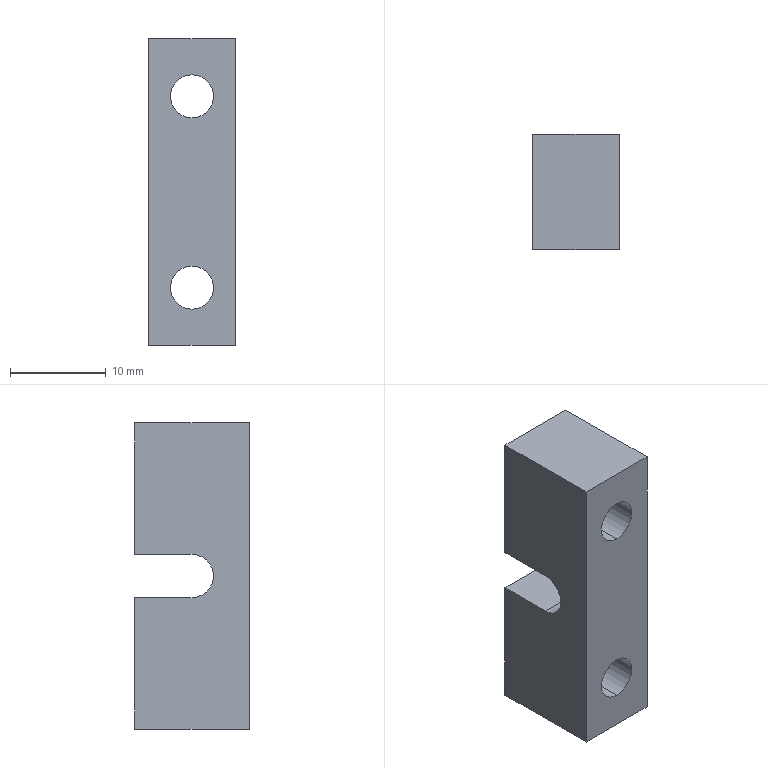Part | STEP file | 001-005-PCB01_5_H6 | 1 solid | 20 faces | box 9 x 12 x 32 mm | volume 2450 mm3 | plane 11 | cylinder 9 | commonest cylinder face diameters 4.5 x5 8 x4
STEP:
#1=CARTESIAN_POINT('',(0.,0.,0.));
#2=DIRECTION('',(0.,0.,1.));
#3=DIRECTION('',(1.,0.,0.));
#4=AXIS2_PLACEMENT_3D('',#1,#2,#3);
#5=CARTESIAN_POINT('',(0.,12.,6.));
#6=VERTEX_POINT('',#5);
#7=CARTESIAN_POINT('',(0.,7.5,6.));
#8=VERTEX_POINT('',#7);
#9=CARTESIAN_POINT('',(0.,12.,6.));
#10=DIRECTION('',(0.,-1.,0.));
#11=VECTOR('',#10,1.);
#12=LINE('',#9,#11);
#13=CARTESIAN_POINT('',(0.,12.,10.));
#14=DIRECTION('',(0.,-1.,0.));
#15=DIRECTION('',(0.,0.,-1.));
#16=AXIS2_PLACEMENT_3D('',#13,#14,#15);
#17=CYLINDRICAL_SURFACE('',#16,4.);
#18=CARTESIAN_POINT('',(6.283,0.));
#19=DIRECTION('',(0.,1.));
#20=VECTOR('',#19,1.);
#21=LINE('',#18,#20);
#22=(GEOMETRIC_REPRESENTATION_CONTEXT(2)PARAMETRIC_REPRESENTATION_CONTEXT()REPRESENTATION_CONTEXT('',''));
#23=DEFINITIONAL_REPRESENTATION('',(#21),#22);
#24=PCURVE('',#17,#23);
#25=CARTESIAN_POINT('',(0.,12.,10.));
#26=DIRECTION('',(0.,-1.,0.));
#27=DIRECTION('',(0.,0.,-1.));
#28=AXIS2_PLACEMENT_3D('',#25,#26,#27);
#29=CYLINDRICAL_SURFACE('',#28,4.);
#30=CARTESIAN_POINT('',(0.,0.));
#31=DIRECTION('',(0.,1.));
#32=VECTOR('',#31,1.);
#33=LINE('',#30,#32);
#34=(GEOMETRIC_REPRESENTATION_CONTEXT(2)PARAMETRIC_REPRESENTATION_CONTEXT()REPRESENTATION_CONTEXT('',''));
#35=DEFINITIONAL_REPRESENTATION('',(#33),#34);
#36=PCURVE('',#29,#35);
#37=SURFACE_CURVE('',#12,(#24,#36),.PCURVE_S1.);
#38=EDGE_CURVE('',#6,#8,#37,.T.);
#39=ORIENTED_EDGE('',*,*,#38,.T.);
#40=CARTESIAN_POINT('',(0.,7.5,14.));
#41=VERTEX_POINT('',#40);
#42=CARTESIAN_POINT('',(0.,7.5,10.));
#43=DIRECTION('',(0.,-1.,0.));
#44=DIRECTION('',(0.,0.,-1.));
#45=AXIS2_PLACEMENT_3D('',#42,#43,#44);
#46=CIRCLE('',#45,4.);
#47=CARTESIAN_POINT('',(0.,4.5));
#48=DIRECTION('',(1.,0.));
#49=VECTOR('',#48,1.);
#50=LINE('',#47,#49);
#51=(GEOMETRIC_REPRESENTATION_CONTEXT(2)PARAMETRIC_REPRESENTATION_CONTEXT()REPRESENTATION_CONTEXT('',''));
#52=DEFINITIONAL_REPRESENTATION('',(#50),#51);
#53=PCURVE('',#17,#52);
#54=CARTESIAN_POINT('',(0.,7.5,12.25));
#55=DIRECTION('',(0.,1.,0.));
#56=DIRECTION('',(0.,0.,1.));
#57=AXIS2_PLACEMENT_3D('',#54,#55,#56);
#58=PLANE('',#57);
#59=CARTESIAN_POINT('',(-6.25,0.));
#60=CARTESIAN_POINT('',(-6.25,6.928));
#61=CARTESIAN_POINT('',(-0.25,3.464));
#62=CARTESIAN_POINT('',(5.75,0.));
#63=CARTESIAN_POINT('',(-0.25,-3.464));
#64=CARTESIAN_POINT('',(-6.25,-6.928));
#65=CARTESIAN_POINT('',(-6.25,0.));
#66=(BOUNDED_CURVE()B_SPLINE_CURVE(2,(#59,#60,#61,#62,#63,#64,#65),.UNSPECIFIED.,.T.,.F.)B_SPLINE_CURVE_WITH_KNOTS((1,2,2,2,2,1),(-2.094,0.,2.094,4.189,6.283,8.378),.UNSPECIFIED.)CURVE()GEOMETRIC_REPRESENTATION_ITEM()RATIONAL_B_SPLINE_CURVE((1.,0.5,1.,0.5,1.,0.5,1.))REPRESENTATION_ITEM(''));
#67=(GEOMETRIC_REPRESENTATION_CONTEXT(2)PARAMETRIC_REPRESENTATION_CONTEXT()REPRESENTATION_CONTEXT('',''));
#68=DEFINITIONAL_REPRESENTATION('',(#66),#67);
#69=PCURVE('',#58,#68);
#70=SURFACE_CURVE('',#46,(#53,#69),.PCURVE_S1.);
#71=EDGE_CURVE('',#41,#8,#70,.T.);
#72=ORIENTED_EDGE('',*,*,#71,.F.);
#73=CARTESIAN_POINT('',(0.,12.,14.));
#74=VERTEX_POINT('',#73);
#75=CARTESIAN_POINT('',(0.,12.,14.));
#76=DIRECTION('',(0.,-1.,0.));
#77=VECTOR('',#76,1.);
#78=LINE('',#75,#77);
#79=CARTESIAN_POINT('',(3.142,0.));
#80=DIRECTION('',(0.,1.));
#81=VECTOR('',#80,1.);
#82=LINE('',#79,#81);
#83=(GEOMETRIC_REPRESENTATION_CONTEXT(2)PARAMETRIC_REPRESENTATION_CONTEXT()REPRESENTATION_CONTEXT('',''));
#84=DEFINITIONAL_REPRESENTATION('',(#82),#83);
#85=PCURVE('',#17,#84);
#86=CARTESIAN_POINT('',(3.142,0.));
#87=DIRECTION('',(0.,1.));
#88=VECTOR('',#87,1.);
#89=LINE('',#86,#88);
#90=(GEOMETRIC_REPRESENTATION_CONTEXT(2)PARAMETRIC_REPRESENTATION_CONTEXT()REPRESENTATION_CONTEXT('',''));
#91=DEFINITIONAL_REPRESENTATION('',(#89),#90);
#92=PCURVE('',#29,#91);
#93=SURFACE_CURVE('',#78,(#85,#92),.PCURVE_S1.);
#94=EDGE_CURVE('',#74,#41,#93,.T.);
#95=ORIENTED_EDGE('',*,*,#94,.F.);
#96=CARTESIAN_POINT('',(0.,12.,10.));
#97=DIRECTION('',(0.,-1.,0.));
#98=DIRECTION('',(0.,0.,-1.));
#99=AXIS2_PLACEMENT_3D('',#96,#97,#98);
#100=CIRCLE('',#99,4.);
#101=CARTESIAN_POINT('',(0.,0.));
#102=DIRECTION('',(1.,0.));
#103=VECTOR('',#102,1.);
#104=LINE('',#101,#103);
#105=(GEOMETRIC_REPRESENTATION_CONTEXT(2)PARAMETRIC_REPRESENTATION_CONTEXT()REPRESENTATION_CONTEXT('',''));
#106=DEFINITIONAL_REPRESENTATION('',(#104),#105);
#107=PCURVE('',#17,#106);
#108=CARTESIAN_POINT('',(4.5,12.,2.25));
#109=DIRECTION('',(0.,-1.,0.));
#110=DIRECTION('',(0.,0.,-1.));
#111=AXIS2_PLACEMENT_3D('',#108,#109,#110);
#112=PLANE('',#111);
#113=CARTESIAN_POINT('',(-7.75,-4.5));
#114=DIRECTION('',(1.,0.));
#115=AXIS2_PLACEMENT_2D('',#113,#114);
#116=CIRCLE('',#115,4.);
#117=(GEOMETRIC_REPRESENTATION_CONTEXT(2)PARAMETRIC_REPRESENTATION_CONTEXT()REPRESENTATION_CONTEXT('',''));
#118=DEFINITIONAL_REPRESENTATION('',(#116),#117);
#119=PCURVE('',#112,#118);
#120=SURFACE_CURVE('',#100,(#107,#119),.PCURVE_S1.);
#121=EDGE_CURVE('',#74,#6,#120,.T.);
#122=ORIENTED_EDGE('',*,*,#121,.T.);
#123=EDGE_LOOP('',(#39,#72,#95,#122));
#124=FACE_BOUND('',#123,.F.);
#125=ADVANCED_FACE('',(#124),#17,.F.);
#126=CARTESIAN_POINT('',(0.,7.5,7.75));
#127=VERTEX_POINT('',#126);
#128=CARTESIAN_POINT('',(0.,0.,7.75));
#129=VERTEX_POINT('',#128);
#130=CARTESIAN_POINT('',(0.,12.,7.75));
#131=DIRECTION('',(0.,-1.,0.));
#132=VECTOR('',#131,1.);
#133=LINE('',#130,#132);
#134=CARTESIAN_POINT('',(0.,12.,10.));
#135=DIRECTION('',(0.,-1.,0.));
#136=DIRECTION('',(0.,0.,-1.));
#137=AXIS2_PLACEMENT_3D('',#134,#135,#136);
#138=CYLINDRICAL_SURFACE('',#137,2.25);
#139=CARTESIAN_POINT('',(6.283,0.));
#140=DIRECTION('',(0.,1.));
#141=VECTOR('',#140,1.);
#142=LINE('',#139,#141);
#143=(GEOMETRIC_REPRESENTATION_CONTEXT(2)PARAMETRIC_REPRESENTATION_CONTEXT()REPRESENTATION_CONTEXT('',''));
#144=DEFINITIONAL_REPRESENTATION('',(#142),#143);
#145=PCURVE('',#138,#144);
#146=CARTESIAN_POINT('',(0.,12.,10.));
#147=DIRECTION('',(0.,-1.,0.));
#148=DIRECTION('',(0.,0.,-1.));
#149=AXIS2_PLACEMENT_3D('',#146,#147,#148);
#150=CYLINDRICAL_SURFACE('',#149,2.25);
#151=CARTESIAN_POINT('',(0.,0.));
#152=DIRECTION('',(0.,1.));
#153=VECTOR('',#152,1.);
#154=LINE('',#151,#153);
#155=(GEOMETRIC_REPRESENTATION_CONTEXT(2)PARAMETRIC_REPRESENTATION_CONTEXT()REPRESENTATION_CONTEXT('',''));
#156=DEFINITIONAL_REPRESENTATION('',(#154),#155);
#157=PCURVE('',#150,#156);
#158=SURFACE_CURVE('',#133,(#145,#157),.PCURVE_S1.);
#159=EDGE_CURVE('',#127,#129,#158,.T.);
#160=ORIENTED_EDGE('',*,*,#159,.T.);
#161=CARTESIAN_POINT('',(0.,0.,12.25));
#162=VERTEX_POINT('',#161);
#163=CARTESIAN_POINT('',(0.,0.,10.));
#164=DIRECTION('',(0.,-1.,0.));
#165=DIRECTION('',(0.,0.,-1.));
#166=AXIS2_PLACEMENT_3D('',#163,#164,#165);
#167=CIRCLE('',#166,2.25);
#168=CARTESIAN_POINT('',(0.,12.));
#169=DIRECTION('',(1.,0.));
#170=VECTOR('',#169,1.);
#171=LINE('',#168,#170);
#172=(GEOMETRIC_REPRESENTATION_CONTEXT(2)PARAMETRIC_REPRESENTATION_CONTEXT()REPRESENTATION_CONTEXT('',''));
#173=DEFINITIONAL_REPRESENTATION('',(#171),#172);
#174=PCURVE('',#138,#173);
#175=CARTESIAN_POINT('',(4.5,0.,16.));
#176=DIRECTION('',(0.,1.,0.));
#177=DIRECTION('',(0.,0.,1.));
#178=AXIS2_PLACEMENT_3D('',#175,#176,#177);
#179=PLANE('',#178);
#180=CARTESIAN_POINT('',(-8.25,-4.5));
#181=CARTESIAN_POINT('',(-8.25,-0.6029));
#182=CARTESIAN_POINT('',(-4.875,-2.551));
#183=CARTESIAN_POINT('',(-1.5,-4.5));
#184=CARTESIAN_POINT('',(-4.875,-6.449));
#185=CARTESIAN_POINT('',(-8.25,-8.397));
#186=CARTESIAN_POINT('',(-8.25,-4.5));
#187=(BOUNDED_CURVE()B_SPLINE_CURVE(2,(#180,#181,#182,#183,#184,#185,#186),.UNSPECIFIED.,.T.,.F.)B_SPLINE_CURVE_WITH_KNOTS((1,2,2,2,2,1),(-2.094,0.,2.094,4.189,6.283,8.378),.UNSPECIFIED.)CURVE()GEOMETRIC_REPRESENTATION_ITEM()RATIONAL_B_SPLINE_CURVE((1.,0.5,1.,0.5,1.,0.5,1.))REPRESENTATION_ITEM(''));
#188=(GEOMETRIC_REPRESENTATION_CONTEXT(2)PARAMETRIC_REPRESENTATION_CONTEXT()REPRESENTATION_CONTEXT('',''));
#189=DEFINITIONAL_REPRESENTATION('',(#187),#188);
#190=PCURVE('',#179,#189);
#191=SURFACE_CURVE('',#167,(#174,#190),.PCURVE_S1.);
#192=EDGE_CURVE('',#162,#129,#191,.T.);
#193=ORIENTED_EDGE('',*,*,#192,.F.);
#194=CARTESIAN_POINT('',(0.,7.5,12.25));
#195=VERTEX_POINT('',#194);
#196=CARTESIAN_POINT('',(0.,12.,12.25));
#197=DIRECTION('',(0.,-1.,0.));
#198=VECTOR('',#197,1.);
#199=LINE('',#196,#198);
#200=CARTESIAN_POINT('',(3.142,0.));
#201=DIRECTION('',(0.,1.));
#202=VECTOR('',#201,1.);
#203=LINE('',#200,#202);
#204=(GEOMETRIC_REPRESENTATION_CONTEXT(2)PARAMETRIC_REPRESENTATION_CONTEXT()REPRESENTATION_CONTEXT('',''));
#205=DEFINITIONAL_REPRESENTATION('',(#203),#204);
#206=PCURVE('',#138,#205);
#207=CARTESIAN_POINT('',(3.142,0.));
#208=DIRECTION('',(0.,1.));
#209=VECTOR('',#208,1.);
#210=LINE('',#207,#209);
#211=(GEOMETRIC_REPRESENTATION_CONTEXT(2)PARAMETRIC_REPRESENTATION_CONTEXT()REPRESENTATION_CONTEXT('',''));
#212=DEFINITIONAL_REPRESENTATION('',(#210),#211);
#213=PCURVE('',#150,#212);
#214=SURFACE_CURVE('',#199,(#206,#213),.PCURVE_S1.);
#215=EDGE_CURVE('',#195,#162,#214,.T.);
#216=ORIENTED_EDGE('',*,*,#215,.F.);
#217=CARTESIAN_POINT('',(0.,7.5,10.));
#218=DIRECTION('',(0.,-1.,0.));
#219=DIRECTION('',(0.,0.,-1.));
#220=AXIS2_PLACEMENT_3D('',#217,#218,#219);
#221=CIRCLE('',#220,2.25);
#222=CARTESIAN_POINT('',(0.,4.5));
#223=DIRECTION('',(1.,0.));
#224=VECTOR('',#223,1.);
#225=LINE('',#222,#224);
#226=(GEOMETRIC_REPRESENTATION_CONTEXT(2)PARAMETRIC_REPRESENTATION_CONTEXT()REPRESENTATION_CONTEXT('',''));
#227=DEFINITIONAL_REPRESENTATION('',(#225),#226);
#228=PCURVE('',#138,#227);
#229=CARTESIAN_POINT('',(-4.5,0.));
#230=CARTESIAN_POINT('',(-4.5,3.897));
#231=CARTESIAN_POINT('',(-1.125,1.949));
#232=CARTESIAN_POINT('',(2.25,0.));
#233=CARTESIAN_POINT('',(-1.125,-1.949));
#234=CARTESIAN_POINT('',(-4.5,-3.897));
#235=CARTESIAN_POINT('',(-4.5,0.));
#236=(BOUNDED_CURVE()B_SPLINE_CURVE(2,(#229,#230,#231,#232,#233,#234,#235),.UNSPECIFIED.,.T.,.F.)B_SPLINE_CURVE_WITH_KNOTS((1,2,2,2,2,1),(-2.094,0.,2.094,4.189,6.283,8.378),.UNSPECIFIED.)CURVE()GEOMETRIC_REPRESENTATION_ITEM()RATIONAL_B_SPLINE_CURVE((1.,0.5,1.,0.5,1.,0.5,1.))REPRESENTATION_ITEM(''));
#237=(GEOMETRIC_REPRESENTATION_CONTEXT(2)PARAMETRIC_REPRESENTATION_CONTEXT()REPRESENTATION_CONTEXT('',''));
#238=DEFINITIONAL_REPRESENTATION('',(#236),#237);
#239=PCURVE('',#58,#238);
#240=SURFACE_CURVE('',#221,(#228,#239),.PCURVE_S1.);
#241=EDGE_CURVE('',#195,#127,#240,.T.);
#242=ORIENTED_EDGE('',*,*,#241,.T.);
#243=EDGE_LOOP('',(#160,#193,#216,#242));
#244=FACE_BOUND('',#243,.F.);
#245=ADVANCED_FACE('',(#244),#138,.F.);
#246=CARTESIAN_POINT('',(0.,12.,-14.));
#247=VERTEX_POINT('',#246);
#248=CARTESIAN_POINT('',(0.,7.5,-14.));
#249=VERTEX_POINT('',#248);
#250=CARTESIAN_POINT('',(0.,12.,-14.));
#251=DIRECTION('',(0.,-1.,0.));
#252=VECTOR('',#251,1.);
#253=LINE('',#250,#252);
#254=CARTESIAN_POINT('',(0.,12.,-10.));
#255=DIRECTION('',(0.,-1.,0.));
#256=DIRECTION('',(0.,0.,-1.));
#257=AXIS2_PLACEMENT_3D('',#254,#255,#256);
#258=CYLINDRICAL_SURFACE('',#257,4.);
#259=CARTESIAN_POINT('',(6.283,0.));
#260=DIRECTION('',(0.,1.));
#261=VECTOR('',#260,1.);
#262=LINE('',#259,#261);
#263=(GEOMETRIC_REPRESENTATION_CONTEXT(2)PARAMETRIC_REPRESENTATION_CONTEXT()REPRESENTATION_CONTEXT('',''));
#264=DEFINITIONAL_REPRESENTATION('',(#262),#263);
#265=PCURVE('',#258,#264);
#266=CARTESIAN_POINT('',(0.,12.,-10.));
#267=DIRECTION('',(0.,-1.,0.));
#268=DIRECTION('',(0.,0.,-1.));
#269=AXIS2_PLACEMENT_3D('',#266,#267,#268);
#270=CYLINDRICAL_SURFACE('',#269,4.);
#271=CARTESIAN_POINT('',(0.,0.));
#272=DIRECTION('',(0.,1.));
#273=VECTOR('',#272,1.);
#274=LINE('',#271,#273);
#275=(GEOMETRIC_REPRESENTATION_CONTEXT(2)PARAMETRIC_REPRESENTATION_CONTEXT()REPRESENTATION_CONTEXT('',''));
#276=DEFINITIONAL_REPRESENTATION('',(#274),#275);
#277=PCURVE('',#270,#276);
#278=SURFACE_CURVE('',#253,(#265,#277),.PCURVE_S1.);
#279=EDGE_CURVE('',#247,#249,#278,.T.);
#280=ORIENTED_EDGE('',*,*,#279,.T.);
#281=CARTESIAN_POINT('',(0.,7.5,-6.));
#282=VERTEX_POINT('',#281);
#283=CARTESIAN_POINT('',(0.,7.5,-10.));
#284=DIRECTION('',(0.,-1.,0.));
#285=DIRECTION('',(0.,0.,-1.));
#286=AXIS2_PLACEMENT_3D('',#283,#284,#285);
#287=CIRCLE('',#286,4.);
#288=CARTESIAN_POINT('',(0.,4.5));
#289=DIRECTION('',(1.,0.));
#290=VECTOR('',#289,1.);
#291=LINE('',#288,#290);
#292=(GEOMETRIC_REPRESENTATION_CONTEXT(2)PARAMETRIC_REPRESENTATION_CONTEXT()REPRESENTATION_CONTEXT('',''));
#293=DEFINITIONAL_REPRESENTATION('',(#291),#292);
#294=PCURVE('',#258,#293);
#295=CARTESIAN_POINT('',(0.,7.5,-7.75));
#296=DIRECTION('',(0.,1.,0.));
#297=DIRECTION('',(0.,0.,1.));
#298=AXIS2_PLACEMENT_3D('',#295,#296,#297);
#299=PLANE('',#298);
#300=CARTESIAN_POINT('',(-6.25,0.));
#301=CARTESIAN_POINT('',(-6.25,6.928));
#302=CARTESIAN_POINT('',(-0.25,3.464));
#303=CARTESIAN_POINT('',(5.75,0.));
#304=CARTESIAN_POINT('',(-0.25,-3.464));
#305=CARTESIAN_POINT('',(-6.25,-6.928));
#306=CARTESIAN_POINT('',(-6.25,0.));
#307=(BOUNDED_CURVE()B_SPLINE_CURVE(2,(#300,#301,#302,#303,#304,#305,#306),.UNSPECIFIED.,.T.,.F.)B_SPLINE_CURVE_WITH_KNOTS((1,2,2,2,2,1),(-2.094,0.,2.094,4.189,6.283,8.378),.UNSPECIFIED.)CURVE()GEOMETRIC_REPRESENTATION_ITEM()RATIONAL_B_SPLINE_CURVE((1.,0.5,1.,0.5,1.,0.5,1.))REPRESENTATION_ITEM(''));
#308=(GEOMETRIC_REPRESENTATION_CONTEXT(2)PARAMETRIC_REPRESENTATION_CONTEXT()REPRESENTATION_CONTEXT('',''));
#309=DEFINITIONAL_REPRESENTATION('',(#307),#308);
#310=PCURVE('',#299,#309);
#311=SURFACE_CURVE('',#287,(#294,#310),.PCURVE_S1.);
#312=EDGE_CURVE('',#282,#249,#311,.T.);
#313=ORIENTED_EDGE('',*,*,#312,.F.);
#314=CARTESIAN_POINT('',(0.,12.,-6.));
#315=VERTEX_POINT('',#314);
#316=CARTESIAN_POINT('',(0.,12.,-6.));
#317=DIRECTION('',(0.,-1.,0.));
#318=VECTOR('',#317,1.);
#319=LINE('',#316,#318);
#320=CARTESIAN_POINT('',(3.142,0.));
#321=DIRECTION('',(0.,1.));
#322=VECTOR('',#321,1.);
#323=LINE('',#320,#322);
#324=(GEOMETRIC_REPRESENTATION_CONTEXT(2)PARAMETRIC_REPRESENTATION_CONTEXT()REPRESENTATION_CONTEXT('',''));
#325=DEFINITIONAL_REPRESENTATION('',(#323),#324);
#326=PCURVE('',#258,#325);
#327=CARTESIAN_POINT('',(3.142,0.));
#328=DIRECTION('',(0.,1.));
#329=VECTOR('',#328,1.);
#330=LINE('',#327,#329);
#331=(GEOMETRIC_REPRESENTATION_CONTEXT(2)PARAMETRIC_REPRESENTATION_CONTEXT()REPRESENTATION_CONTEXT('',''));
#332=DEFINITIONAL_REPRESENTATION('',(#330),#331);
#333=PCURVE('',#270,#332);
#334=SURFACE_CURVE('',#319,(#326,#333),.PCURVE_S1.);
#335=EDGE_CURVE('',#315,#282,#334,.T.);
#336=ORIENTED_EDGE('',*,*,#335,.F.);
#337=CARTESIAN_POINT('',(0.,12.,-10.));
#338=DIRECTION('',(0.,-1.,0.));
#339=DIRECTION('',(0.,0.,-1.));
#340=AXIS2_PLACEMENT_3D('',#337,#338,#339);
#341=CIRCLE('',#340,4.);
#342=CARTESIAN_POINT('',(0.,0.));
#343=DIRECTION('',(1.,0.));
#344=VECTOR('',#343,1.);
#345=LINE('',#342,#344);
#346=(GEOMETRIC_REPRESENTATION_CONTEXT(2)PARAMETRIC_REPRESENTATION_CONTEXT()REPRESENTATION_CONTEXT('',''));
#347=DEFINITIONAL_REPRESENTATION('',(#345),#346);
#348=PCURVE('',#258,#347);
#349=CARTESIAN_POINT('',(4.5,12.,-16.));
#350=DIRECTION('',(0.,-1.,0.));
#351=DIRECTION('',(0.,0.,-1.));
#352=AXIS2_PLACEMENT_3D('',#349,#350,#351);
#353=PLANE('',#352);
#354=CARTESIAN_POINT('',(-6.,-4.5));
#355=DIRECTION('',(1.,0.));
#356=AXIS2_PLACEMENT_2D('',#354,#355);
#357=CIRCLE('',#356,4.);
#358=(GEOMETRIC_REPRESENTATION_CONTEXT(2)PARAMETRIC_REPRESENTATION_CONTEXT()REPRESENTATION_CONTEXT('',''));
#359=DEFINITIONAL_REPRESENTATION('',(#357),#358);
#360=PCURVE('',#353,#359);
#361=SURFACE_CURVE('',#341,(#348,#360),.PCURVE_S1.);
#362=EDGE_CURVE('',#315,#247,#361,.T.);
#363=ORIENTED_EDGE('',*,*,#362,.T.);
#364=EDGE_LOOP('',(#280,#313,#336,#363));
#365=FACE_BOUND('',#364,.F.);
#366=ADVANCED_FACE('',(#365),#258,.F.);
#367=CARTESIAN_POINT('',(0.,7.5,-12.25));
#368=VERTEX_POINT('',#367);
#369=CARTESIAN_POINT('',(0.,0.,-12.25));
#370=VERTEX_POINT('',#369);
#371=CARTESIAN_POINT('',(0.,12.,-12.25));
#372=DIRECTION('',(0.,-1.,0.));
#373=VECTOR('',#372,1.);
#374=LINE('',#371,#373);
#375=CARTESIAN_POINT('',(0.,12.,-10.));
#376=DIRECTION('',(0.,-1.,0.));
#377=DIRECTION('',(0.,0.,-1.));
#378=AXIS2_PLACEMENT_3D('',#375,#376,#377);
#379=CYLINDRICAL_SURFACE('',#378,2.25);
#380=CARTESIAN_POINT('',(6.283,0.));
#381=DIRECTION('',(0.,1.));
#382=VECTOR('',#381,1.);
#383=LINE('',#380,#382);
#384=(GEOMETRIC_REPRESENTATION_CONTEXT(2)PARAMETRIC_REPRESENTATION_CONTEXT()REPRESENTATION_CONTEXT('',''));
#385=DEFINITIONAL_REPRESENTATION('',(#383),#384);
#386=PCURVE('',#379,#385);
#387=CARTESIAN_POINT('',(0.,12.,-10.));
#388=DIRECTION('',(0.,-1.,0.));
#389=DIRECTION('',(0.,0.,-1.));
#390=AXIS2_PLACEMENT_3D('',#387,#388,#389);
#391=CYLINDRICAL_SURFACE('',#390,2.25);
#392=CARTESIAN_POINT('',(0.,0.));
#393=DIRECTION('',(0.,1.));
#394=VECTOR('',#393,1.);
#395=LINE('',#392,#394);
#396=(GEOMETRIC_REPRESENTATION_CONTEXT(2)PARAMETRIC_REPRESENTATION_CONTEXT()REPRESENTATION_CONTEXT('',''));
#397=DEFINITIONAL_REPRESENTATION('',(#395),#396);
#398=PCURVE('',#391,#397);
#399=SURFACE_CURVE('',#374,(#386,#398),.PCURVE_S1.);
#400=EDGE_CURVE('',#368,#370,#399,.T.);
#401=ORIENTED_EDGE('',*,*,#400,.T.);
#402=CARTESIAN_POINT('',(0.,0.,-7.75));
#403=VERTEX_POINT('',#402);
#404=CARTESIAN_POINT('',(0.,0.,-10.));
#405=DIRECTION('',(0.,-1.,0.));
#406=DIRECTION('',(0.,0.,-1.));
#407=AXIS2_PLACEMENT_3D('',#404,#405,#406);
#408=CIRCLE('',#407,2.25);
#409=CARTESIAN_POINT('',(0.,12.));
#410=DIRECTION('',(1.,0.));
#411=VECTOR('',#410,1.);
#412=LINE('',#409,#411);
#413=(GEOMETRIC_REPRESENTATION_CONTEXT(2)PARAMETRIC_REPRESENTATION_CONTEXT()REPRESENTATION_CONTEXT('',''));
#414=DEFINITIONAL_REPRESENTATION('',(#412),#413);
#415=PCURVE('',#379,#414);
#416=CARTESIAN_POINT('',(-28.25,-4.5));
#417=CARTESIAN_POINT('',(-28.25,-0.6029));
#418=CARTESIAN_POINT('',(-24.875,-2.551));
#419=CARTESIAN_POINT('',(-21.5,-4.5));
#420=CARTESIAN_POINT('',(-24.875,-6.449));
#421=CARTESIAN_POINT('',(-28.25,-8.397));
#422=CARTESIAN_POINT('',(-28.25,-4.5));
#423=(BOUNDED_CURVE()B_SPLINE_CURVE(2,(#416,#417,#418,#419,#420,#421,#422),.UNSPECIFIED.,.T.,.F.)B_SPLINE_CURVE_WITH_KNOTS((1,2,2,2,2,1),(-2.094,0.,2.094,4.189,6.283,8.378),.UNSPECIFIED.)CURVE()GEOMETRIC_REPRESENTATION_ITEM()RATIONAL_B_SPLINE_CURVE((1.,0.5,1.,0.5,1.,0.5,1.))REPRESENTATION_ITEM(''));
#424=(GEOMETRIC_REPRESENTATION_CONTEXT(2)PARAMETRIC_REPRESENTATION_CONTEXT()REPRESENTATION_CONTEXT('',''));
#425=DEFINITIONAL_REPRESENTATION('',(#423),#424);
#426=PCURVE('',#179,#425);
#427=SURFACE_CURVE('',#408,(#415,#426),.PCURVE_S1.);
#428=EDGE_CURVE('',#403,#370,#427,.T.);
#429=ORIENTED_EDGE('',*,*,#428,.F.);
#430=CARTESIAN_POINT('',(0.,7.5,-7.75));
#431=VERTEX_POINT('',#430);
#432=CARTESIAN_POINT('',(0.,12.,-7.75));
#433=DIRECTION('',(0.,-1.,0.));
#434=VECTOR('',#433,1.);
#435=LINE('',#432,#434);
#436=CARTESIAN_POINT('',(3.142,0.));
#437=DIRECTION('',(0.,1.));
#438=VECTOR('',#437,1.);
#439=LINE('',#436,#438);
#440=(GEOMETRIC_REPRESENTATION_CONTEXT(2)PARAMETRIC_REPRESENTATION_CONTEXT()REPRESENTATION_CONTEXT('',''));
#441=DEFINITIONAL_REPRESENTATION('',(#439),#440);
#442=PCURVE('',#379,#441);
#443=CARTESIAN_POINT('',(3.142,0.));
#444=DIRECTION('',(0.,1.));
#445=VECTOR('',#444,1.);
#446=LINE('',#443,#445);
#447=(GEOMETRIC_REPRESENTATION_CONTEXT(2)PARAMETRIC_REPRESENTATION_CONTEXT()REPRESENTATION_CONTEXT('',''));
#448=DEFINITIONAL_REPRESENTATION('',(#446),#447);
#449=PCURVE('',#391,#448);
#450=SURFACE_CURVE('',#435,(#442,#449),.PCURVE_S1.);
#451=EDGE_CURVE('',#431,#403,#450,.T.);
#452=ORIENTED_EDGE('',*,*,#451,.F.);
#453=CARTESIAN_POINT('',(0.,7.5,-10.));
#454=DIRECTION('',(0.,-1.,0.));
#455=DIRECTION('',(0.,0.,-1.));
#456=AXIS2_PLACEMENT_3D('',#453,#454,#455);
#457=CIRCLE('',#456,2.25);
#458=CARTESIAN_POINT('',(0.,4.5));
#459=DIRECTION('',(1.,0.));
#460=VECTOR('',#459,1.);
#461=LINE('',#458,#460);
#462=(GEOMETRIC_REPRESENTATION_CONTEXT(2)PARAMETRIC_REPRESENTATION_CONTEXT()REPRESENTATION_CONTEXT('',''));
#463=DEFINITIONAL_REPRESENTATION('',(#461),#462);
#464=PCURVE('',#379,#463);
#465=CARTESIAN_POINT('',(-4.5,0.));
#466=CARTESIAN_POINT('',(-4.5,3.897));
#467=CARTESIAN_POINT('',(-1.125,1.949));
#468=CARTESIAN_POINT('',(2.25,0.));
#469=CARTESIAN_POINT('',(-1.125,-1.949));
#470=CARTESIAN_POINT('',(-4.5,-3.897));
#471=CARTESIAN_POINT('',(-4.5,0.));
#472=(BOUNDED_CURVE()B_SPLINE_CURVE(2,(#465,#466,#467,#468,#469,#470,#471),.UNSPECIFIED.,.T.,.F.)B_SPLINE_CURVE_WITH_KNOTS((1,2,2,2,2,1),(-2.094,0.,2.094,4.189,6.283,8.378),.UNSPECIFIED.)CURVE()GEOMETRIC_REPRESENTATION_ITEM()RATIONAL_B_SPLINE_CURVE((1.,0.5,1.,0.5,1.,0.5,1.))REPRESENTATION_ITEM(''));
#473=(GEOMETRIC_REPRESENTATION_CONTEXT(2)PARAMETRIC_REPRESENTATION_CONTEXT()REPRESENTATION_CONTEXT('',''));
#474=DEFINITIONAL_REPRESENTATION('',(#472),#473);
#475=PCURVE('',#299,#474);
#476=SURFACE_CURVE('',#457,(#464,#475),.PCURVE_S1.);
#477=EDGE_CURVE('',#431,#368,#476,.T.);
#478=ORIENTED_EDGE('',*,*,#477,.T.);
#479=EDGE_LOOP('',(#401,#429,#452,#478));
#480=FACE_BOUND('',#479,.F.);
#481=ADVANCED_FACE('',(#480),#379,.F.);
#482=CARTESIAN_POINT('',(0.,12.,10.));
#483=DIRECTION('',(0.,-1.,0.));
#484=DIRECTION('',(0.,0.,-1.));
#485=AXIS2_PLACEMENT_3D('',#482,#483,#484);
#486=CIRCLE('',#485,4.);
#487=CARTESIAN_POINT('',(-7.75,-4.5));
#488=DIRECTION('',(1.,0.));
#489=AXIS2_PLACEMENT_2D('',#487,#488);
#490=CIRCLE('',#489,4.);
#491=(GEOMETRIC_REPRESENTATION_CONTEXT(2)PARAMETRIC_REPRESENTATION_CONTEXT()REPRESENTATION_CONTEXT('',''));
#492=DEFINITIONAL_REPRESENTATION('',(#490),#491);
#493=PCURVE('',#112,#492);
#494=CARTESIAN_POINT('',(0.,0.));
#495=DIRECTION('',(1.,0.));
#496=VECTOR('',#495,1.);
#497=LINE('',#494,#496);
#498=(GEOMETRIC_REPRESENTATION_CONTEXT(2)PARAMETRIC_REPRESENTATION_CONTEXT()REPRESENTATION_CONTEXT('',''));
#499=DEFINITIONAL_REPRESENTATION('',(#497),#498);
#500=PCURVE('',#29,#499);
#501=SURFACE_CURVE('',#486,(#493,#500),.PCURVE_S1.);
#502=EDGE_CURVE('',#6,#74,#501,.T.);
#503=ORIENTED_EDGE('',*,*,#502,.T.);
#504=ORIENTED_EDGE('',*,*,#121,.T.);
#505=EDGE_LOOP('',(#503,#504));
#506=FACE_BOUND('',#505,.T.);
#507=CARTESIAN_POINT('',(4.5,12.,2.25));
#508=VERTEX_POINT('',#507);
#509=CARTESIAN_POINT('',(-4.5,12.,2.25));
#510=VERTEX_POINT('',#509);
#511=CARTESIAN_POINT('',(4.5,12.,2.25));
#512=DIRECTION('',(-1.,0.,0.));
#513=VECTOR('',#512,1.);
#514=LINE('',#511,#513);
#515=CARTESIAN_POINT('',(0.,0.));
#516=DIRECTION('',(0.,-1.));
#517=VECTOR('',#516,1.);
#518=LINE('',#515,#517);
#519=(GEOMETRIC_REPRESENTATION_CONTEXT(2)PARAMETRIC_REPRESENTATION_CONTEXT()REPRESENTATION_CONTEXT('',''));
#520=DEFINITIONAL_REPRESENTATION('',(#518),#519);
#521=PCURVE('',#112,#520);
#522=CARTESIAN_POINT('',(4.5,6.,2.25));
#523=DIRECTION('',(0.,0.,1.));
#524=DIRECTION('',(1.,0.,0.));
#525=AXIS2_PLACEMENT_3D('',#522,#523,#524);
#526=PLANE('',#525);
#527=CARTESIAN_POINT('',(0.,6.));
#528=DIRECTION('',(-1.,0.));
#529=VECTOR('',#528,1.);
#530=LINE('',#527,#529);
#531=(GEOMETRIC_REPRESENTATION_CONTEXT(2)PARAMETRIC_REPRESENTATION_CONTEXT()REPRESENTATION_CONTEXT('',''));
#532=DEFINITIONAL_REPRESENTATION('',(#530),#531);
#533=PCURVE('',#526,#532);
#534=SURFACE_CURVE('',#514,(#521,#533),.PCURVE_S1.);
#535=EDGE_CURVE('',#508,#510,#534,.T.);
#536=ORIENTED_EDGE('',*,*,#535,.T.);
#537=CARTESIAN_POINT('',(-4.5,12.,16.));
#538=VERTEX_POINT('',#537);
#539=CARTESIAN_POINT('',(-4.5,12.,2.25));
#540=DIRECTION('',(0.,0.,1.));
#541=VECTOR('',#540,1.);
#542=LINE('',#539,#541);
#543=CARTESIAN_POINT('',(0.,-9.));
#544=DIRECTION('',(-1.,0.));
#545=VECTOR('',#544,1.);
#546=LINE('',#543,#545);
#547=(GEOMETRIC_REPRESENTATION_CONTEXT(2)PARAMETRIC_REPRESENTATION_CONTEXT()REPRESENTATION_CONTEXT('',''));
#548=DEFINITIONAL_REPRESENTATION('',(#546),#547);
#549=PCURVE('',#112,#548);
#550=CARTESIAN_POINT('',(-4.5,6.,0.));
#551=DIRECTION('',(-1.,0.,0.));
#552=DIRECTION('',(0.,0.,1.));
#553=AXIS2_PLACEMENT_3D('',#550,#551,#552);
#554=PLANE('',#553);
#555=CARTESIAN_POINT('',(2.25,6.));
#556=DIRECTION('',(1.,0.));
#557=VECTOR('',#556,1.);
#558=LINE('',#555,#557);
#559=(GEOMETRIC_REPRESENTATION_CONTEXT(2)PARAMETRIC_REPRESENTATION_CONTEXT()REPRESENTATION_CONTEXT('',''));
#560=DEFINITIONAL_REPRESENTATION('',(#558),#559);
#561=PCURVE('',#554,#560);
#562=SURFACE_CURVE('',#542,(#549,#561),.PCURVE_S1.);
#563=EDGE_CURVE('',#510,#538,#562,.T.);
#564=ORIENTED_EDGE('',*,*,#563,.T.);
#565=CARTESIAN_POINT('',(4.5,12.,16.));
#566=VERTEX_POINT('',#565);
#567=CARTESIAN_POINT('',(4.5,12.,16.));
#568=DIRECTION('',(-1.,0.,0.));
#569=VECTOR('',#568,1.);
#570=LINE('',#567,#569);
#571=CARTESIAN_POINT('',(-13.75,0.));
#572=DIRECTION('',(0.,-1.));
#573=VECTOR('',#572,1.);
#574=LINE('',#571,#573);
#575=(GEOMETRIC_REPRESENTATION_CONTEXT(2)PARAMETRIC_REPRESENTATION_CONTEXT()REPRESENTATION_CONTEXT('',''));
#576=DEFINITIONAL_REPRESENTATION('',(#574),#575);
#577=PCURVE('',#112,#576);
#578=CARTESIAN_POINT('',(4.5,12.,16.));
#579=DIRECTION('',(0.,0.,-1.));
#580=DIRECTION('',(-1.,0.,0.));
#581=AXIS2_PLACEMENT_3D('',#578,#579,#580);
#582=PLANE('',#581);
#583=CARTESIAN_POINT('',(0.,0.));
#584=DIRECTION('',(1.,0.));
#585=VECTOR('',#584,1.);
#586=LINE('',#583,#585);
#587=(GEOMETRIC_REPRESENTATION_CONTEXT(2)PARAMETRIC_REPRESENTATION_CONTEXT()REPRESENTATION_CONTEXT('',''));
#588=DEFINITIONAL_REPRESENTATION('',(#586),#587);
#589=PCURVE('',#582,#588);
#590=SURFACE_CURVE('',#570,(#577,#589),.PCURVE_S1.);
#591=EDGE_CURVE('',#566,#538,#590,.T.);
#592=ORIENTED_EDGE('',*,*,#591,.F.);
#593=CARTESIAN_POINT('',(4.5,12.,2.25));
#594=DIRECTION('',(0.,0.,1.));
#595=VECTOR('',#594,1.);
#596=LINE('',#593,#595);
#597=CARTESIAN_POINT('',(0.,0.));
#598=DIRECTION('',(-1.,0.));
#599=VECTOR('',#598,1.);
#600=LINE('',#597,#599);
#601=(GEOMETRIC_REPRESENTATION_CONTEXT(2)PARAMETRIC_REPRESENTATION_CONTEXT()REPRESENTATION_CONTEXT('',''));
#602=DEFINITIONAL_REPRESENTATION('',(#600),#601);
#603=PCURVE('',#112,#602);
#604=CARTESIAN_POINT('',(4.5,6.,0.));
#605=DIRECTION('',(-1.,0.,0.));
#606=DIRECTION('',(0.,0.,1.));
#607=AXIS2_PLACEMENT_3D('',#604,#605,#606);
#608=PLANE('',#607);
#609=CARTESIAN_POINT('',(2.25,6.));
#610=DIRECTION('',(1.,0.));
#611=VECTOR('',#610,1.);
#612=LINE('',#609,#611);
#613=(GEOMETRIC_REPRESENTATION_CONTEXT(2)PARAMETRIC_REPRESENTATION_CONTEXT()REPRESENTATION_CONTEXT('',''));
#614=DEFINITIONAL_REPRESENTATION('',(#612),#613);
#615=PCURVE('',#608,#614);
#616=SURFACE_CURVE('',#596,(#603,#615),.PCURVE_S1.);
#617=EDGE_CURVE('',#508,#566,#616,.T.);
#618=ORIENTED_EDGE('',*,*,#617,.F.);
#619=EDGE_LOOP('',(#536,#564,#592,#618));
#620=FACE_BOUND('',#619,.T.);
#621=ADVANCED_FACE('',(#506,#620),#112,.F.);
#622=ORIENTED_EDGE('',*,*,#591,.T.);
#623=CARTESIAN_POINT('',(-4.5,0.,16.));
#624=VERTEX_POINT('',#623);
#625=CARTESIAN_POINT('',(-4.5,12.,16.));
#626=DIRECTION('',(0.,-1.,0.));
#627=VECTOR('',#626,1.);
#628=LINE('',#625,#627);
#629=CARTESIAN_POINT('',(9.,0.));
#630=DIRECTION('',(0.,-1.));
#631=VECTOR('',#630,1.);
#632=LINE('',#629,#631);
#633=(GEOMETRIC_REPRESENTATION_CONTEXT(2)PARAMETRIC_REPRESENTATION_CONTEXT()REPRESENTATION_CONTEXT('',''));
#634=DEFINITIONAL_REPRESENTATION('',(#632),#633);
#635=PCURVE('',#582,#634);
#636=CARTESIAN_POINT('',(16.,6.));
#637=DIRECTION('',(0.,-1.));
#638=VECTOR('',#637,1.);
#639=LINE('',#636,#638);
#640=(GEOMETRIC_REPRESENTATION_CONTEXT(2)PARAMETRIC_REPRESENTATION_CONTEXT()REPRESENTATION_CONTEXT('',''));
#641=DEFINITIONAL_REPRESENTATION('',(#639),#640);
#642=PCURVE('',#554,#641);
#643=SURFACE_CURVE('',#628,(#635,#642),.PCURVE_S1.);
#644=EDGE_CURVE('',#538,#624,#643,.T.);
#645=ORIENTED_EDGE('',*,*,#644,.T.);
#646=CARTESIAN_POINT('',(4.5,0.,16.));
#647=VERTEX_POINT('',#646);
#648=CARTESIAN_POINT('',(4.5,0.,16.));
#649=DIRECTION('',(-1.,0.,0.));
#650=VECTOR('',#649,1.);
#651=LINE('',#648,#650);
#652=CARTESIAN_POINT('',(0.,-12.));
#653=DIRECTION('',(1.,0.));
#654=VECTOR('',#653,1.);
#655=LINE('',#652,#654);
#656=(GEOMETRIC_REPRESENTATION_CONTEXT(2)PARAMETRIC_REPRESENTATION_CONTEXT()REPRESENTATION_CONTEXT('',''));
#657=DEFINITIONAL_REPRESENTATION('',(#655),#656);
#658=PCURVE('',#582,#657);
#659=CARTESIAN_POINT('',(0.,0.));
#660=DIRECTION('',(0.,-1.));
#661=VECTOR('',#660,1.);
#662=LINE('',#659,#661);
#663=(GEOMETRIC_REPRESENTATION_CONTEXT(2)PARAMETRIC_REPRESENTATION_CONTEXT()REPRESENTATION_CONTEXT('',''));
#664=DEFINITIONAL_REPRESENTATION('',(#662),#663);
#665=PCURVE('',#179,#664);
#666=SURFACE_CURVE('',#651,(#658,#665),.PCURVE_S1.);
#667=EDGE_CURVE('',#647,#624,#666,.T.);
#668=ORIENTED_EDGE('',*,*,#667,.F.);
#669=CARTESIAN_POINT('',(4.5,12.,16.));
#670=DIRECTION('',(0.,-1.,0.));
#671=VECTOR('',#670,1.);
#672=LINE('',#669,#671);
#673=CARTESIAN_POINT('',(0.,0.));
#674=DIRECTION('',(0.,-1.));
#675=VECTOR('',#674,1.);
#676=LINE('',#673,#675);
#677=(GEOMETRIC_REPRESENTATION_CONTEXT(2)PARAMETRIC_REPRESENTATION_CONTEXT()REPRESENTATION_CONTEXT('',''));
#678=DEFINITIONAL_REPRESENTATION('',(#676),#677);
#679=PCURVE('',#582,#678);
#680=CARTESIAN_POINT('',(16.,6.));
#681=DIRECTION('',(0.,-1.));
#682=VECTOR('',#681,1.);
#683=LINE('',#680,#682);
#684=(GEOMETRIC_REPRESENTATION_CONTEXT(2)PARAMETRIC_REPRESENTATION_CONTEXT()REPRESENTATION_CONTEXT('',''));
#685=DEFINITIONAL_REPRESENTATION('',(#683),#684);
#686=PCURVE('',#608,#685);
#687=SURFACE_CURVE('',#672,(#679,#686),.PCURVE_S1.);
#688=EDGE_CURVE('',#566,#647,#687,.T.);
#689=ORIENTED_EDGE('',*,*,#688,.F.);
#690=EDGE_LOOP('',(#622,#645,#668,#689));
#691=FACE_BOUND('',#690,.T.);
#692=ADVANCED_FACE('',(#691),#582,.F.);
#693=CARTESIAN_POINT('',(0.,0.,10.));
#694=DIRECTION('',(0.,-1.,0.));
#695=DIRECTION('',(0.,0.,-1.));
#696=AXIS2_PLACEMENT_3D('',#693,#694,#695);
#697=CIRCLE('',#696,2.25);
#698=CARTESIAN_POINT('',(-8.25,-4.5));
#699=CARTESIAN_POINT('',(-8.25,-0.6029));
#700=CARTESIAN_POINT('',(-4.875,-2.551));
#701=CARTESIAN_POINT('',(-1.5,-4.5));
#702=CARTESIAN_POINT('',(-4.875,-6.449));
#703=CARTESIAN_POINT('',(-8.25,-8.397));
#704=CARTESIAN_POINT('',(-8.25,-4.5));
#705=(BOUNDED_CURVE()B_SPLINE_CURVE(2,(#698,#699,#700,#701,#702,#703,#704),.UNSPECIFIED.,.T.,.F.)B_SPLINE_CURVE_WITH_KNOTS((1,2,2,2,2,1),(-2.094,0.,2.094,4.189,6.283,8.378),.UNSPECIFIED.)CURVE()GEOMETRIC_REPRESENTATION_ITEM()RATIONAL_B_SPLINE_CURVE((1.,0.5,1.,0.5,1.,0.5,1.))REPRESENTATION_ITEM(''));
#706=(GEOMETRIC_REPRESENTATION_CONTEXT(2)PARAMETRIC_REPRESENTATION_CONTEXT()REPRESENTATION_CONTEXT('',''));
#707=DEFINITIONAL_REPRESENTATION('',(#705),#706);
#708=PCURVE('',#179,#707);
#709=CARTESIAN_POINT('',(0.,12.));
#710=DIRECTION('',(1.,0.));
#711=VECTOR('',#710,1.);
#712=LINE('',#709,#711);
#713=(GEOMETRIC_REPRESENTATION_CONTEXT(2)PARAMETRIC_REPRESENTATION_CONTEXT()REPRESENTATION_CONTEXT('',''));
#714=DEFINITIONAL_REPRESENTATION('',(#712),#713);
#715=PCURVE('',#150,#714);
#716=SURFACE_CURVE('',#697,(#708,#715),.PCURVE_S1.);
#717=EDGE_CURVE('',#129,#162,#716,.T.);
#718=ORIENTED_EDGE('',*,*,#717,.F.);
#719=ORIENTED_EDGE('',*,*,#192,.F.);
#720=EDGE_LOOP('',(#718,#719));
#721=FACE_BOUND('',#720,.T.);
#722=CARTESIAN_POINT('',(0.,0.,-10.));
#723=DIRECTION('',(0.,-1.,0.));
#724=DIRECTION('',(0.,0.,-1.));
#725=AXIS2_PLACEMENT_3D('',#722,#723,#724);
#726=CIRCLE('',#725,2.25);
#727=CARTESIAN_POINT('',(-28.25,-4.5));
#728=CARTESIAN_POINT('',(-28.25,-0.6029));
#729=CARTESIAN_POINT('',(-24.875,-2.551));
#730=CARTESIAN_POINT('',(-21.5,-4.5));
#731=CARTESIAN_POINT('',(-24.875,-6.449));
#732=CARTESIAN_POINT('',(-28.25,-8.397));
#733=CARTESIAN_POINT('',(-28.25,-4.5));
#734=(BOUNDED_CURVE()B_SPLINE_CURVE(2,(#727,#728,#729,#730,#731,#732,#733),.UNSPECIFIED.,.T.,.F.)B_SPLINE_CURVE_WITH_KNOTS((1,2,2,2,2,1),(-2.094,0.,2.094,4.189,6.283,8.378),.UNSPECIFIED.)CURVE()GEOMETRIC_REPRESENTATION_ITEM()RATIONAL_B_SPLINE_CURVE((1.,0.5,1.,0.5,1.,0.5,1.))REPRESENTATION_ITEM(''));
#735=(GEOMETRIC_REPRESENTATION_CONTEXT(2)PARAMETRIC_REPRESENTATION_CONTEXT()REPRESENTATION_CONTEXT('',''));
#736=DEFINITIONAL_REPRESENTATION('',(#734),#735);
#737=PCURVE('',#179,#736);
#738=CARTESIAN_POINT('',(0.,12.));
#739=DIRECTION('',(1.,0.));
#740=VECTOR('',#739,1.);
#741=LINE('',#738,#740);
#742=(GEOMETRIC_REPRESENTATION_CONTEXT(2)PARAMETRIC_REPRESENTATION_CONTEXT()REPRESENTATION_CONTEXT('',''));
#743=DEFINITIONAL_REPRESENTATION('',(#741),#742);
#744=PCURVE('',#391,#743);
#745=SURFACE_CURVE('',#726,(#737,#744),.PCURVE_S1.);
#746=EDGE_CURVE('',#370,#403,#745,.T.);
#747=ORIENTED_EDGE('',*,*,#746,.F.);
#748=ORIENTED_EDGE('',*,*,#428,.F.);
#749=EDGE_LOOP('',(#747,#748));
#750=FACE_BOUND('',#749,.T.);
#751=ORIENTED_EDGE('',*,*,#667,.T.);
#752=CARTESIAN_POINT('',(-4.5,0.,-16.));
#753=VERTEX_POINT('',#752);
#754=CARTESIAN_POINT('',(-4.5,0.,16.));
#755=DIRECTION('',(0.,0.,-1.));
#756=VECTOR('',#755,1.);
#757=LINE('',#754,#756);
#758=CARTESIAN_POINT('',(0.,-9.));
#759=DIRECTION('',(-1.,0.));
#760=VECTOR('',#759,1.);
#761=LINE('',#758,#760);
#762=(GEOMETRIC_REPRESENTATION_CONTEXT(2)PARAMETRIC_REPRESENTATION_CONTEXT()REPRESENTATION_CONTEXT('',''));
#763=DEFINITIONAL_REPRESENTATION('',(#761),#762);
#764=PCURVE('',#179,#763);
#765=CARTESIAN_POINT('',(16.,-6.));
#766=DIRECTION('',(-1.,0.));
#767=VECTOR('',#766,1.);
#768=LINE('',#765,#767);
#769=(GEOMETRIC_REPRESENTATION_CONTEXT(2)PARAMETRIC_REPRESENTATION_CONTEXT()REPRESENTATION_CONTEXT('',''));
#770=DEFINITIONAL_REPRESENTATION('',(#768),#769);
#771=PCURVE('',#554,#770);
#772=SURFACE_CURVE('',#757,(#764,#771),.PCURVE_S1.);
#773=EDGE_CURVE('',#624,#753,#772,.T.);
#774=ORIENTED_EDGE('',*,*,#773,.T.);
#775=CARTESIAN_POINT('',(4.5,0.,-16.));
#776=VERTEX_POINT('',#775);
#777=CARTESIAN_POINT('',(4.5,0.,-16.));
#778=DIRECTION('',(-1.,0.,0.));
#779=VECTOR('',#778,1.);
#780=LINE('',#777,#779);
#781=CARTESIAN_POINT('',(-32.,0.));
#782=DIRECTION('',(0.,-1.));
#783=VECTOR('',#782,1.);
#784=LINE('',#781,#783);
#785=(GEOMETRIC_REPRESENTATION_CONTEXT(2)PARAMETRIC_REPRESENTATION_CONTEXT()REPRESENTATION_CONTEXT('',''));
#786=DEFINITIONAL_REPRESENTATION('',(#784),#785);
#787=PCURVE('',#179,#786);
#788=CARTESIAN_POINT('',(4.5,0.,-16.));
#789=DIRECTION('',(0.,0.,1.));
#790=DIRECTION('',(1.,0.,0.));
#791=AXIS2_PLACEMENT_3D('',#788,#789,#790);
#792=PLANE('',#791);
#793=CARTESIAN_POINT('',(0.,0.));
#794=DIRECTION('',(-1.,0.));
#795=VECTOR('',#794,1.);
#796=LINE('',#793,#795);
#797=(GEOMETRIC_REPRESENTATION_CONTEXT(2)PARAMETRIC_REPRESENTATION_CONTEXT()REPRESENTATION_CONTEXT('',''));
#798=DEFINITIONAL_REPRESENTATION('',(#796),#797);
#799=PCURVE('',#792,#798);
#800=SURFACE_CURVE('',#780,(#787,#799),.PCURVE_S1.);
#801=EDGE_CURVE('',#776,#753,#800,.T.);
#802=ORIENTED_EDGE('',*,*,#801,.F.);
#803=CARTESIAN_POINT('',(4.5,0.,16.));
#804=DIRECTION('',(0.,0.,-1.));
#805=VECTOR('',#804,1.);
#806=LINE('',#803,#805);
#807=CARTESIAN_POINT('',(0.,0.));
#808=DIRECTION('',(-1.,0.));
#809=VECTOR('',#808,1.);
#810=LINE('',#807,#809);
#811=(GEOMETRIC_REPRESENTATION_CONTEXT(2)PARAMETRIC_REPRESENTATION_CONTEXT()REPRESENTATION_CONTEXT('',''));
#812=DEFINITIONAL_REPRESENTATION('',(#810),#811);
#813=PCURVE('',#179,#812);
#814=CARTESIAN_POINT('',(16.,-6.));
#815=DIRECTION('',(-1.,0.));
#816=VECTOR('',#815,1.);
#817=LINE('',#814,#816);
#818=(GEOMETRIC_REPRESENTATION_CONTEXT(2)PARAMETRIC_REPRESENTATION_CONTEXT()REPRESENTATION_CONTEXT('',''));
#819=DEFINITIONAL_REPRESENTATION('',(#817),#818);
#820=PCURVE('',#608,#819);
#821=SURFACE_CURVE('',#806,(#813,#820),.PCURVE_S1.);
#822=EDGE_CURVE('',#647,#776,#821,.T.);
#823=ORIENTED_EDGE('',*,*,#822,.F.);
#824=EDGE_LOOP('',(#751,#774,#802,#823));
#825=FACE_BOUND('',#824,.T.);
#826=ADVANCED_FACE('',(#721,#750,#825),#179,.F.);
#827=ORIENTED_EDGE('',*,*,#801,.T.);
#828=CARTESIAN_POINT('',(-4.5,12.,-16.));
#829=VERTEX_POINT('',#828);
#830=CARTESIAN_POINT('',(-4.5,0.,-16.));
#831=DIRECTION('',(0.,1.,0.));
#832=VECTOR('',#831,1.);
#833=LINE('',#830,#832);
#834=CARTESIAN_POINT('',(-9.,0.));
#835=DIRECTION('',(0.,1.));
#836=VECTOR('',#835,1.);
#837=LINE('',#834,#836);
#838=(GEOMETRIC_REPRESENTATION_CONTEXT(2)PARAMETRIC_REPRESENTATION_CONTEXT()REPRESENTATION_CONTEXT('',''));
#839=DEFINITIONAL_REPRESENTATION('',(#837),#838);
#840=PCURVE('',#792,#839);
#841=CARTESIAN_POINT('',(-16.,-6.));
#842=DIRECTION('',(0.,1.));
#843=VECTOR('',#842,1.);
#844=LINE('',#841,#843);
#845=(GEOMETRIC_REPRESENTATION_CONTEXT(2)PARAMETRIC_REPRESENTATION_CONTEXT()REPRESENTATION_CONTEXT('',''));
#846=DEFINITIONAL_REPRESENTATION('',(#844),#845);
#847=PCURVE('',#554,#846);
#848=SURFACE_CURVE('',#833,(#840,#847),.PCURVE_S1.);
#849=EDGE_CURVE('',#753,#829,#848,.T.);
#850=ORIENTED_EDGE('',*,*,#849,.T.);
#851=CARTESIAN_POINT('',(4.5,12.,-16.));
#852=VERTEX_POINT('',#851);
#853=CARTESIAN_POINT('',(4.5,12.,-16.));
#854=DIRECTION('',(-1.,0.,0.));
#855=VECTOR('',#854,1.);
#856=LINE('',#853,#855);
#857=CARTESIAN_POINT('',(0.,12.));
#858=DIRECTION('',(-1.,0.));
#859=VECTOR('',#858,1.);
#860=LINE('',#857,#859);
#861=(GEOMETRIC_REPRESENTATION_CONTEXT(2)PARAMETRIC_REPRESENTATION_CONTEXT()REPRESENTATION_CONTEXT('',''));
#862=DEFINITIONAL_REPRESENTATION('',(#860),#861);
#863=PCURVE('',#792,#862);
#864=CARTESIAN_POINT('',(0.,0.));
#865=DIRECTION('',(0.,-1.));
#866=VECTOR('',#865,1.);
#867=LINE('',#864,#866);
#868=(GEOMETRIC_REPRESENTATION_CONTEXT(2)PARAMETRIC_REPRESENTATION_CONTEXT()REPRESENTATION_CONTEXT('',''));
#869=DEFINITIONAL_REPRESENTATION('',(#867),#868);
#870=PCURVE('',#353,#869);
#871=SURFACE_CURVE('',#856,(#863,#870),.PCURVE_S1.);
#872=EDGE_CURVE('',#852,#829,#871,.T.);
#873=ORIENTED_EDGE('',*,*,#872,.F.);
#874=CARTESIAN_POINT('',(4.5,0.,-16.));
#875=DIRECTION('',(0.,1.,0.));
#876=VECTOR('',#875,1.);
#877=LINE('',#874,#876);
#878=CARTESIAN_POINT('',(0.,0.));
#879=DIRECTION('',(0.,1.));
#880=VECTOR('',#879,1.);
#881=LINE('',#878,#880);
#882=(GEOMETRIC_REPRESENTATION_CONTEXT(2)PARAMETRIC_REPRESENTATION_CONTEXT()REPRESENTATION_CONTEXT('',''));
#883=DEFINITIONAL_REPRESENTATION('',(#881),#882);
#884=PCURVE('',#792,#883);
#885=CARTESIAN_POINT('',(-16.,-6.));
#886=DIRECTION('',(0.,1.));
#887=VECTOR('',#886,1.);
#888=LINE('',#885,#887);
#889=(GEOMETRIC_REPRESENTATION_CONTEXT(2)PARAMETRIC_REPRESENTATION_CONTEXT()REPRESENTATION_CONTEXT('',''));
#890=DEFINITIONAL_REPRESENTATION('',(#888),#889);
#891=PCURVE('',#608,#890);
#892=SURFACE_CURVE('',#877,(#884,#891),.PCURVE_S1.);
#893=EDGE_CURVE('',#776,#852,#892,.T.);
#894=ORIENTED_EDGE('',*,*,#893,.F.);
#895=EDGE_LOOP('',(#827,#850,#873,#894));
#896=FACE_BOUND('',#895,.T.);
#897=ADVANCED_FACE('',(#896),#792,.F.);
#898=CARTESIAN_POINT('',(0.,12.,-10.));
#899=DIRECTION('',(0.,-1.,0.));
#900=DIRECTION('',(0.,0.,-1.));
#901=AXIS2_PLACEMENT_3D('',#898,#899,#900);
#902=CIRCLE('',#901,4.);
#903=CARTESIAN_POINT('',(-6.,-4.5));
#904=DIRECTION('',(1.,0.));
#905=AXIS2_PLACEMENT_2D('',#903,#904);
#906=CIRCLE('',#905,4.);
#907=(GEOMETRIC_REPRESENTATION_CONTEXT(2)PARAMETRIC_REPRESENTATION_CONTEXT()REPRESENTATION_CONTEXT('',''));
#908=DEFINITIONAL_REPRESENTATION('',(#906),#907);
#909=PCURVE('',#353,#908);
#910=CARTESIAN_POINT('',(0.,0.));
#911=DIRECTION('',(1.,0.));
#912=VECTOR('',#911,1.);
#913=LINE('',#910,#912);
#914=(GEOMETRIC_REPRESENTATION_CONTEXT(2)PARAMETRIC_REPRESENTATION_CONTEXT()REPRESENTATION_CONTEXT('',''));
#915=DEFINITIONAL_REPRESENTATION('',(#913),#914);
#916=PCURVE('',#270,#915);
#917=SURFACE_CURVE('',#902,(#909,#916),.PCURVE_S1.);
#918=EDGE_CURVE('',#247,#315,#917,.T.);
#919=ORIENTED_EDGE('',*,*,#918,.T.);
#920=ORIENTED_EDGE('',*,*,#362,.T.);
#921=EDGE_LOOP('',(#919,#920));
#922=FACE_BOUND('',#921,.T.);
#923=ORIENTED_EDGE('',*,*,#872,.T.);
#924=CARTESIAN_POINT('',(-4.5,12.,-2.25));
#925=VERTEX_POINT('',#924);
#926=CARTESIAN_POINT('',(-4.5,12.,-16.));
#927=DIRECTION('',(0.,0.,1.));
#928=VECTOR('',#927,1.);
#929=LINE('',#926,#928);
#930=CARTESIAN_POINT('',(0.,-9.));
#931=DIRECTION('',(-1.,0.));
#932=VECTOR('',#931,1.);
#933=LINE('',#930,#932);
#934=(GEOMETRIC_REPRESENTATION_CONTEXT(2)PARAMETRIC_REPRESENTATION_CONTEXT()REPRESENTATION_CONTEXT('',''));
#935=DEFINITIONAL_REPRESENTATION('',(#933),#934);
#936=PCURVE('',#353,#935);
#937=CARTESIAN_POINT('',(-16.,6.));
#938=DIRECTION('',(1.,0.));
#939=VECTOR('',#938,1.);
#940=LINE('',#937,#939);
#941=(GEOMETRIC_REPRESENTATION_CONTEXT(2)PARAMETRIC_REPRESENTATION_CONTEXT()REPRESENTATION_CONTEXT('',''));
#942=DEFINITIONAL_REPRESENTATION('',(#940),#941);
#943=PCURVE('',#554,#942);
#944=SURFACE_CURVE('',#929,(#936,#943),.PCURVE_S1.);
#945=EDGE_CURVE('',#829,#925,#944,.T.);
#946=ORIENTED_EDGE('',*,*,#945,.T.);
#947=CARTESIAN_POINT('',(4.5,12.,-2.25));
#948=VERTEX_POINT('',#947);
#949=CARTESIAN_POINT('',(4.5,12.,-2.25));
#950=DIRECTION('',(-1.,0.,0.));
#951=VECTOR('',#950,1.);
#952=LINE('',#949,#951);
#953=CARTESIAN_POINT('',(-13.75,0.));
#954=DIRECTION('',(0.,-1.));
#955=VECTOR('',#954,1.);
#956=LINE('',#953,#955);
#957=(GEOMETRIC_REPRESENTATION_CONTEXT(2)PARAMETRIC_REPRESENTATION_CONTEXT()REPRESENTATION_CONTEXT('',''));
#958=DEFINITIONAL_REPRESENTATION('',(#956),#957);
#959=PCURVE('',#353,#958);
#960=CARTESIAN_POINT('',(4.5,12.,-2.25));
#961=DIRECTION('',(0.,0.,-1.));
#962=DIRECTION('',(-1.,0.,0.));
#963=AXIS2_PLACEMENT_3D('',#960,#961,#962);
#964=PLANE('',#963);
#965=CARTESIAN_POINT('',(0.,0.));
#966=DIRECTION('',(1.,0.));
#967=VECTOR('',#966,1.);
#968=LINE('',#965,#967);
#969=(GEOMETRIC_REPRESENTATION_CONTEXT(2)PARAMETRIC_REPRESENTATION_CONTEXT()REPRESENTATION_CONTEXT('',''));
#970=DEFINITIONAL_REPRESENTATION('',(#968),#969);
#971=PCURVE('',#964,#970);
#972=SURFACE_CURVE('',#952,(#959,#971),.PCURVE_S1.);
#973=EDGE_CURVE('',#948,#925,#972,.T.);
#974=ORIENTED_EDGE('',*,*,#973,.F.);
#975=CARTESIAN_POINT('',(4.5,12.,-16.));
#976=DIRECTION('',(0.,0.,1.));
#977=VECTOR('',#976,1.);
#978=LINE('',#975,#977);
#979=CARTESIAN_POINT('',(0.,0.));
#980=DIRECTION('',(-1.,0.));
#981=VECTOR('',#980,1.);
#982=LINE('',#979,#981);
#983=(GEOMETRIC_REPRESENTATION_CONTEXT(2)PARAMETRIC_REPRESENTATION_CONTEXT()REPRESENTATION_CONTEXT('',''));
#984=DEFINITIONAL_REPRESENTATION('',(#982),#983);
#985=PCURVE('',#353,#984);
#986=CARTESIAN_POINT('',(-16.,6.));
#987=DIRECTION('',(1.,0.));
#988=VECTOR('',#987,1.);
#989=LINE('',#986,#988);
#990=(GEOMETRIC_REPRESENTATION_CONTEXT(2)PARAMETRIC_REPRESENTATION_CONTEXT()REPRESENTATION_CONTEXT('',''));
#991=DEFINITIONAL_REPRESENTATION('',(#989),#990);
#992=PCURVE('',#608,#991);
#993=SURFACE_CURVE('',#978,(#985,#992),.PCURVE_S1.);
#994=EDGE_CURVE('',#852,#948,#993,.T.);
#995=ORIENTED_EDGE('',*,*,#994,.F.);
#996=EDGE_LOOP('',(#923,#946,#974,#995));
#997=FACE_BOUND('',#996,.T.);
#998=ADVANCED_FACE('',(#922,#997),#353,.F.);
#999=ORIENTED_EDGE('',*,*,#973,.T.);
#1000=CARTESIAN_POINT('',(-4.5,6.,-2.25));
#1001=VERTEX_POINT('',#1000);
#1002=CARTESIAN_POINT('',(-4.5,12.,-2.25));
#1003=DIRECTION('',(0.,-1.,0.));
#1004=VECTOR('',#1003,1.);
#1005=LINE('',#1002,#1004);
#1006=CARTESIAN_POINT('',(9.,0.));
#1007=DIRECTION('',(0.,-1.));
#1008=VECTOR('',#1007,1.);
#1009=LINE('',#1006,#1008);
#1010=(GEOMETRIC_REPRESENTATION_CONTEXT(2)PARAMETRIC_REPRESENTATION_CONTEXT()REPRESENTATION_CONTEXT('',''));
#1011=DEFINITIONAL_REPRESENTATION('',(#1009),#1010);
#1012=PCURVE('',#964,#1011);
#1013=CARTESIAN_POINT('',(-2.25,6.));
#1014=DIRECTION('',(0.,-1.));
#1015=VECTOR('',#1014,1.);
#1016=LINE('',#1013,#1015);
#1017=(GEOMETRIC_REPRESENTATION_CONTEXT(2)PARAMETRIC_REPRESENTATION_CONTEXT()REPRESENTATION_CONTEXT('',''));
#1018=DEFINITIONAL_REPRESENTATION('',(#1016),#1017);
#1019=PCURVE('',#554,#1018);
#1020=SURFACE_CURVE('',#1005,(#1012,#1019),.PCURVE_S1.);
#1021=EDGE_CURVE('',#925,#1001,#1020,.T.);
#1022=ORIENTED_EDGE('',*,*,#1021,.T.);
#1023=CARTESIAN_POINT('',(4.5,6.,-2.25));
#1024=VERTEX_POINT('',#1023);
#1025=CARTESIAN_POINT('',(4.5,6.,-2.25));
#1026=DIRECTION('',(-1.,0.,0.));
#1027=VECTOR('',#1026,1.);
#1028=LINE('',#1025,#1027);
#1029=CARTESIAN_POINT('',(0.,-6.));
#1030=DIRECTION('',(1.,0.));
#1031=VECTOR('',#1030,1.);
#1032=LINE('',#1029,#1031);
#1033=(GEOMETRIC_REPRESENTATION_CONTEXT(2)PARAMETRIC_REPRESENTATION_CONTEXT()REPRESENTATION_CONTEXT('',''));
#1034=DEFINITIONAL_REPRESENTATION('',(#1032),#1033);
#1035=PCURVE('',#964,#1034);
#1036=CARTESIAN_POINT('',(4.5,6.,0.));
#1037=DIRECTION('',(-1.,0.,0.));
#1038=DIRECTION('',(0.,0.,1.));
#1039=AXIS2_PLACEMENT_3D('',#1036,#1037,#1038);
#1040=CYLINDRICAL_SURFACE('',#1039,2.25);
#1041=CARTESIAN_POINT('',(3.142,0.));
#1042=DIRECTION('',(0.,1.));
#1043=VECTOR('',#1042,1.);
#1044=LINE('',#1041,#1043);
#1045=(GEOMETRIC_REPRESENTATION_CONTEXT(2)PARAMETRIC_REPRESENTATION_CONTEXT()REPRESENTATION_CONTEXT('',''));
#1046=DEFINITIONAL_REPRESENTATION('',(#1044),#1045);
#1047=PCURVE('',#1040,#1046);
#1048=SURFACE_CURVE('',#1028,(#1035,#1047),.PCURVE_S1.);
#1049=EDGE_CURVE('',#1024,#1001,#1048,.T.);
#1050=ORIENTED_EDGE('',*,*,#1049,.F.);
#1051=CARTESIAN_POINT('',(4.5,12.,-2.25));
#1052=DIRECTION('',(0.,-1.,0.));
#1053=VECTOR('',#1052,1.);
#1054=LINE('',#1051,#1053);
#1055=CARTESIAN_POINT('',(0.,0.));
#1056=DIRECTION('',(0.,-1.));
#1057=VECTOR('',#1056,1.);
#1058=LINE('',#1055,#1057);
#1059=(GEOMETRIC_REPRESENTATION_CONTEXT(2)PARAMETRIC_REPRESENTATION_CONTEXT()REPRESENTATION_CONTEXT('',''));
#1060=DEFINITIONAL_REPRESENTATION('',(#1058),#1059);
#1061=PCURVE('',#964,#1060);
#1062=CARTESIAN_POINT('',(-2.25,6.));
#1063=DIRECTION('',(0.,-1.));
#1064=VECTOR('',#1063,1.);
#1065=LINE('',#1062,#1064);
#1066=(GEOMETRIC_REPRESENTATION_CONTEXT(2)PARAMETRIC_REPRESENTATION_CONTEXT()REPRESENTATION_CONTEXT('',''));
#1067=DEFINITIONAL_REPRESENTATION('',(#1065),#1066);
#1068=PCURVE('',#608,#1067);
#1069=SURFACE_CURVE('',#1054,(#1061,#1068),.PCURVE_S1.);
#1070=EDGE_CURVE('',#948,#1024,#1069,.T.);
#1071=ORIENTED_EDGE('',*,*,#1070,.F.);
#1072=EDGE_LOOP('',(#999,#1022,#1050,#1071));
#1073=FACE_BOUND('',#1072,.T.);
#1074=ADVANCED_FACE('',(#1073),#964,.F.);
#1075=CARTESIAN_POINT('',(4.5,6.,2.25));
#1076=VERTEX_POINT('',#1075);
#1077=CARTESIAN_POINT('',(4.5,6.,0.));
#1078=DIRECTION('',(-1.,0.,0.));
#1079=DIRECTION('',(0.,0.,1.));
#1080=AXIS2_PLACEMENT_3D('',#1077,#1078,#1079);
#1081=CIRCLE('',#1080,2.25);
#1082=CARTESIAN_POINT('',(0.,0.));
#1083=DIRECTION('',(1.,0.));
#1084=VECTOR('',#1083,1.);
#1085=LINE('',#1082,#1084);
#1086=(GEOMETRIC_REPRESENTATION_CONTEXT(2)PARAMETRIC_REPRESENTATION_CONTEXT()REPRESENTATION_CONTEXT('',''));
#1087=DEFINITIONAL_REPRESENTATION('',(#1085),#1086);
#1088=PCURVE('',#1040,#1087);
#1089=CARTESIAN_POINT('',(0.,0.));
#1090=DIRECTION('',(1.,0.));
#1091=AXIS2_PLACEMENT_2D('',#1089,#1090);
#1092=CIRCLE('',#1091,2.25);
#1093=(GEOMETRIC_REPRESENTATION_CONTEXT(2)PARAMETRIC_REPRESENTATION_CONTEXT()REPRESENTATION_CONTEXT('',''));
#1094=DEFINITIONAL_REPRESENTATION('',(#1092),#1093);
#1095=PCURVE('',#608,#1094);
#1096=SURFACE_CURVE('',#1081,(#1088,#1095),.PCURVE_S1.);
#1097=EDGE_CURVE('',#1024,#1076,#1096,.T.);
#1098=ORIENTED_EDGE('',*,*,#1097,.T.);
#1099=CARTESIAN_POINT('',(-4.5,6.,2.25));
#1100=VERTEX_POINT('',#1099);
#1101=CARTESIAN_POINT('',(4.5,6.,2.25));
#1102=DIRECTION('',(-1.,0.,0.));
#1103=VECTOR('',#1102,1.);
#1104=LINE('',#1101,#1103);
#1105=CARTESIAN_POINT('',(6.283,0.));
#1106=DIRECTION('',(0.,1.));
#1107=VECTOR('',#1106,1.);
#1108=LINE('',#1105,#1107);
#1109=(GEOMETRIC_REPRESENTATION_CONTEXT(2)PARAMETRIC_REPRESENTATION_CONTEXT()REPRESENTATION_CONTEXT('',''));
#1110=DEFINITIONAL_REPRESENTATION('',(#1108),#1109);
#1111=PCURVE('',#1040,#1110);
#1112=CARTESIAN_POINT('',(0.,0.));
#1113=DIRECTION('',(-1.,0.));
#1114=VECTOR('',#1113,1.);
#1115=LINE('',#1112,#1114);
#1116=(GEOMETRIC_REPRESENTATION_CONTEXT(2)PARAMETRIC_REPRESENTATION_CONTEXT()REPRESENTATION_CONTEXT('',''));
#1117=DEFINITIONAL_REPRESENTATION('',(#1115),#1116);
#1118=PCURVE('',#526,#1117);
#1119=SURFACE_CURVE('',#1104,(#1111,#1118),.PCURVE_S1.);
#1120=EDGE_CURVE('',#1076,#1100,#1119,.T.);
#1121=ORIENTED_EDGE('',*,*,#1120,.T.);
#1122=CARTESIAN_POINT('',(-4.5,6.,0.));
#1123=DIRECTION('',(-1.,0.,0.));
#1124=DIRECTION('',(0.,0.,1.));
#1125=AXIS2_PLACEMENT_3D('',#1122,#1123,#1124);
#1126=CIRCLE('',#1125,2.25);
#1127=CARTESIAN_POINT('',(0.,9.));
#1128=DIRECTION('',(1.,0.));
#1129=VECTOR('',#1128,1.);
#1130=LINE('',#1127,#1129);
#1131=(GEOMETRIC_REPRESENTATION_CONTEXT(2)PARAMETRIC_REPRESENTATION_CONTEXT()REPRESENTATION_CONTEXT('',''));
#1132=DEFINITIONAL_REPRESENTATION('',(#1130),#1131);
#1133=PCURVE('',#1040,#1132);
#1134=CARTESIAN_POINT('',(0.,0.));
#1135=DIRECTION('',(1.,0.));
#1136=AXIS2_PLACEMENT_2D('',#1134,#1135);
#1137=CIRCLE('',#1136,2.25);
#1138=(GEOMETRIC_REPRESENTATION_CONTEXT(2)PARAMETRIC_REPRESENTATION_CONTEXT()REPRESENTATION_CONTEXT('',''));
#1139=DEFINITIONAL_REPRESENTATION('',(#1137),#1138);
#1140=PCURVE('',#554,#1139);
#1141=SURFACE_CURVE('',#1126,(#1133,#1140),.PCURVE_S1.);
#1142=EDGE_CURVE('',#1001,#1100,#1141,.T.);
#1143=ORIENTED_EDGE('',*,*,#1142,.F.);
#1144=ORIENTED_EDGE('',*,*,#1049,.F.);
#1145=EDGE_LOOP('',(#1098,#1121,#1143,#1144));
#1146=FACE_BOUND('',#1145,.F.);
#1147=ADVANCED_FACE('',(#1146),#1040,.F.);
#1148=ORIENTED_EDGE('',*,*,#1120,.T.);
#1149=CARTESIAN_POINT('',(-4.5,6.,2.25));
#1150=DIRECTION('',(0.,1.,0.));
#1151=VECTOR('',#1150,1.);
#1152=LINE('',#1149,#1151);
#1153=CARTESIAN_POINT('',(-9.,0.));
#1154=DIRECTION('',(0.,1.));
#1155=VECTOR('',#1154,1.);
#1156=LINE('',#1153,#1155);
#1157=(GEOMETRIC_REPRESENTATION_CONTEXT(2)PARAMETRIC_REPRESENTATION_CONTEXT()REPRESENTATION_CONTEXT('',''));
#1158=DEFINITIONAL_REPRESENTATION('',(#1156),#1157);
#1159=PCURVE('',#526,#1158);
#1160=CARTESIAN_POINT('',(2.25,0.));
#1161=DIRECTION('',(0.,1.));
#1162=VECTOR('',#1161,1.);
#1163=LINE('',#1160,#1162);
#1164=(GEOMETRIC_REPRESENTATION_CONTEXT(2)PARAMETRIC_REPRESENTATION_CONTEXT()REPRESENTATION_CONTEXT('',''));
#1165=DEFINITIONAL_REPRESENTATION('',(#1163),#1164);
#1166=PCURVE('',#554,#1165);
#1167=SURFACE_CURVE('',#1152,(#1159,#1166),.PCURVE_S1.);
#1168=EDGE_CURVE('',#1100,#510,#1167,.T.);
#1169=ORIENTED_EDGE('',*,*,#1168,.T.);
#1170=ORIENTED_EDGE('',*,*,#535,.F.);
#1171=CARTESIAN_POINT('',(4.5,6.,2.25));
#1172=DIRECTION('',(0.,1.,0.));
#1173=VECTOR('',#1172,1.);
#1174=LINE('',#1171,#1173);
#1175=CARTESIAN_POINT('',(0.,0.));
#1176=DIRECTION('',(0.,1.));
#1177=VECTOR('',#1176,1.);
#1178=LINE('',#1175,#1177);
#1179=(GEOMETRIC_REPRESENTATION_CONTEXT(2)PARAMETRIC_REPRESENTATION_CONTEXT()REPRESENTATION_CONTEXT('',''));
#1180=DEFINITIONAL_REPRESENTATION('',(#1178),#1179);
#1181=PCURVE('',#526,#1180);
#1182=CARTESIAN_POINT('',(2.25,0.));
#1183=DIRECTION('',(0.,1.));
#1184=VECTOR('',#1183,1.);
#1185=LINE('',#1182,#1184);
#1186=(GEOMETRIC_REPRESENTATION_CONTEXT(2)PARAMETRIC_REPRESENTATION_CONTEXT()REPRESENTATION_CONTEXT('',''));
#1187=DEFINITIONAL_REPRESENTATION('',(#1185),#1186);
#1188=PCURVE('',#608,#1187);
#1189=SURFACE_CURVE('',#1174,(#1181,#1188),.PCURVE_S1.);
#1190=EDGE_CURVE('',#1076,#508,#1189,.T.);
#1191=ORIENTED_EDGE('',*,*,#1190,.F.);
#1192=EDGE_LOOP('',(#1148,#1169,#1170,#1191));
#1193=FACE_BOUND('',#1192,.T.);
#1194=ADVANCED_FACE('',(#1193),#526,.F.);
#1195=ORIENTED_EDGE('',*,*,#617,.T.);
#1196=ORIENTED_EDGE('',*,*,#688,.T.);
#1197=ORIENTED_EDGE('',*,*,#822,.T.);
#1198=ORIENTED_EDGE('',*,*,#893,.T.);
#1199=ORIENTED_EDGE('',*,*,#994,.T.);
#1200=ORIENTED_EDGE('',*,*,#1070,.T.);
#1201=ORIENTED_EDGE('',*,*,#1097,.T.);
#1202=ORIENTED_EDGE('',*,*,#1190,.T.);
#1203=EDGE_LOOP('',(#1195,#1196,#1197,#1198,#1199,#1200,#1201,#1202));
#1204=FACE_BOUND('',#1203,.T.);
#1205=ADVANCED_FACE('',(#1204),#608,.F.);
#1206=ORIENTED_EDGE('',*,*,#563,.F.);
#1207=ORIENTED_EDGE('',*,*,#1168,.F.);
#1208=ORIENTED_EDGE('',*,*,#1142,.F.);
#1209=ORIENTED_EDGE('',*,*,#1021,.F.);
#1210=ORIENTED_EDGE('',*,*,#945,.F.);
#1211=ORIENTED_EDGE('',*,*,#849,.F.);
#1212=ORIENTED_EDGE('',*,*,#773,.F.);
#1213=ORIENTED_EDGE('',*,*,#644,.F.);
#1214=EDGE_LOOP('',(#1206,#1207,#1208,#1209,#1210,#1211,#1212,#1213));
#1215=FACE_BOUND('',#1214,.T.);
#1216=ADVANCED_FACE('',(#1215),#554,.T.);
#1217=ORIENTED_EDGE('',*,*,#746,.F.);
#1218=ORIENTED_EDGE('',*,*,#400,.F.);
#1219=CARTESIAN_POINT('',(0.,7.5,-10.));
#1220=DIRECTION('',(0.,-1.,0.));
#1221=DIRECTION('',(0.,0.,-1.));
#1222=AXIS2_PLACEMENT_3D('',#1219,#1220,#1221);
#1223=CIRCLE('',#1222,2.25);
#1224=CARTESIAN_POINT('',(0.,4.5));
#1225=DIRECTION('',(1.,0.));
#1226=VECTOR('',#1225,1.);
#1227=LINE('',#1224,#1226);
#1228=(GEOMETRIC_REPRESENTATION_CONTEXT(2)PARAMETRIC_REPRESENTATION_CONTEXT()REPRESENTATION_CONTEXT('',''));
#1229=DEFINITIONAL_REPRESENTATION('',(#1227),#1228);
#1230=PCURVE('',#391,#1229);
#1231=CARTESIAN_POINT('',(-4.5,0.));
#1232=CARTESIAN_POINT('',(-4.5,3.897));
#1233=CARTESIAN_POINT('',(-1.125,1.949));
#1234=CARTESIAN_POINT('',(2.25,0.));
#1235=CARTESIAN_POINT('',(-1.125,-1.949));
#1236=CARTESIAN_POINT('',(-4.5,-3.897));
#1237=CARTESIAN_POINT('',(-4.5,0.));
#1238=(BOUNDED_CURVE()B_SPLINE_CURVE(2,(#1231,#1232,#1233,#1234,#1235,#1236,#1237),.UNSPECIFIED.,.T.,.F.)B_SPLINE_CURVE_WITH_KNOTS((1,2,2,2,2,1),(-2.094,0.,2.094,4.189,6.283,8.378),.UNSPECIFIED.)CURVE()GEOMETRIC_REPRESENTATION_ITEM()RATIONAL_B_SPLINE_CURVE((1.,0.5,1.,0.5,1.,0.5,1.))REPRESENTATION_ITEM(''));
#1239=(GEOMETRIC_REPRESENTATION_CONTEXT(2)PARAMETRIC_REPRESENTATION_CONTEXT()REPRESENTATION_CONTEXT('',''));
#1240=DEFINITIONAL_REPRESENTATION('',(#1238),#1239);
#1241=PCURVE('',#299,#1240);
#1242=SURFACE_CURVE('',#1223,(#1230,#1241),.PCURVE_S1.);
#1243=EDGE_CURVE('',#368,#431,#1242,.T.);
#1244=ORIENTED_EDGE('',*,*,#1243,.T.);
#1245=ORIENTED_EDGE('',*,*,#451,.T.);
#1246=EDGE_LOOP('',(#1217,#1218,#1244,#1245));
#1247=FACE_BOUND('',#1246,.F.);
#1248=ADVANCED_FACE('',(#1247),#391,.F.);
#1249=ORIENTED_EDGE('',*,*,#1243,.T.);
#1250=ORIENTED_EDGE('',*,*,#477,.T.);
#1251=EDGE_LOOP('',(#1249,#1250));
#1252=FACE_BOUND('',#1251,.T.);
#1253=CARTESIAN_POINT('',(0.,7.5,-10.));
#1254=DIRECTION('',(0.,-1.,0.));
#1255=DIRECTION('',(0.,0.,-1.));
#1256=AXIS2_PLACEMENT_3D('',#1253,#1254,#1255);
#1257=CIRCLE('',#1256,4.);
#1258=CARTESIAN_POINT('',(-6.25,0.));
#1259=CARTESIAN_POINT('',(-6.25,6.928));
#1260=CARTESIAN_POINT('',(-0.25,3.464));
#1261=CARTESIAN_POINT('',(5.75,0.));
#1262=CARTESIAN_POINT('',(-0.25,-3.464));
#1263=CARTESIAN_POINT('',(-6.25,-6.928));
#1264=CARTESIAN_POINT('',(-6.25,0.));
#1265=(BOUNDED_CURVE()B_SPLINE_CURVE(2,(#1258,#1259,#1260,#1261,#1262,#1263,#1264),.UNSPECIFIED.,.T.,.F.)B_SPLINE_CURVE_WITH_KNOTS((1,2,2,2,2,1),(-2.094,0.,2.094,4.189,6.283,8.378),.UNSPECIFIED.)CURVE()GEOMETRIC_REPRESENTATION_ITEM()RATIONAL_B_SPLINE_CURVE((1.,0.5,1.,0.5,1.,0.5,1.))REPRESENTATION_ITEM(''));
#1266=(GEOMETRIC_REPRESENTATION_CONTEXT(2)PARAMETRIC_REPRESENTATION_CONTEXT()REPRESENTATION_CONTEXT('',''));
#1267=DEFINITIONAL_REPRESENTATION('',(#1265),#1266);
#1268=PCURVE('',#299,#1267);
#1269=CARTESIAN_POINT('',(0.,4.5));
#1270=DIRECTION('',(1.,0.));
#1271=VECTOR('',#1270,1.);
#1272=LINE('',#1269,#1271);
#1273=(GEOMETRIC_REPRESENTATION_CONTEXT(2)PARAMETRIC_REPRESENTATION_CONTEXT()REPRESENTATION_CONTEXT('',''));
#1274=DEFINITIONAL_REPRESENTATION('',(#1272),#1273);
#1275=PCURVE('',#270,#1274);
#1276=SURFACE_CURVE('',#1257,(#1268,#1275),.PCURVE_S1.);
#1277=EDGE_CURVE('',#249,#282,#1276,.T.);
#1278=ORIENTED_EDGE('',*,*,#1277,.F.);
#1279=ORIENTED_EDGE('',*,*,#312,.F.);
#1280=EDGE_LOOP('',(#1278,#1279));
#1281=FACE_BOUND('',#1280,.T.);
#1282=ADVANCED_FACE('',(#1252,#1281),#299,.T.);
#1283=ORIENTED_EDGE('',*,*,#1277,.F.);
#1284=ORIENTED_EDGE('',*,*,#279,.F.);
#1285=ORIENTED_EDGE('',*,*,#918,.T.);
#1286=ORIENTED_EDGE('',*,*,#335,.T.);
#1287=EDGE_LOOP('',(#1283,#1284,#1285,#1286));
#1288=FACE_BOUND('',#1287,.F.);
#1289=ADVANCED_FACE('',(#1288),#270,.F.);
#1290=ORIENTED_EDGE('',*,*,#717,.F.);
#1291=ORIENTED_EDGE('',*,*,#159,.F.);
#1292=CARTESIAN_POINT('',(0.,7.5,10.));
#1293=DIRECTION('',(0.,-1.,0.));
#1294=DIRECTION('',(0.,0.,-1.));
#1295=AXIS2_PLACEMENT_3D('',#1292,#1293,#1294);
#1296=CIRCLE('',#1295,2.25);
#1297=CARTESIAN_POINT('',(0.,4.5));
#1298=DIRECTION('',(1.,0.));
#1299=VECTOR('',#1298,1.);
#1300=LINE('',#1297,#1299);
#1301=(GEOMETRIC_REPRESENTATION_CONTEXT(2)PARAMETRIC_REPRESENTATION_CONTEXT()REPRESENTATION_CONTEXT('',''));
#1302=DEFINITIONAL_REPRESENTATION('',(#1300),#1301);
#1303=PCURVE('',#150,#1302);
#1304=CARTESIAN_POINT('',(-4.5,0.));
#1305=CARTESIAN_POINT('',(-4.5,3.897));
#1306=CARTESIAN_POINT('',(-1.125,1.949));
#1307=CARTESIAN_POINT('',(2.25,0.));
#1308=CARTESIAN_POINT('',(-1.125,-1.949));
#1309=CARTESIAN_POINT('',(-4.5,-3.897));
#1310=CARTESIAN_POINT('',(-4.5,0.));
#1311=(BOUNDED_CURVE()B_SPLINE_CURVE(2,(#1304,#1305,#1306,#1307,#1308,#1309,#1310),.UNSPECIFIED.,.T.,.F.)B_SPLINE_CURVE_WITH_KNOTS((1,2,2,2,2,1),(-2.094,0.,2.094,4.189,6.283,8.378),.UNSPECIFIED.)CURVE()GEOMETRIC_REPRESENTATION_ITEM()RATIONAL_B_SPLINE_CURVE((1.,0.5,1.,0.5,1.,0.5,1.))REPRESENTATION_ITEM(''));
#1312=(GEOMETRIC_REPRESENTATION_CONTEXT(2)PARAMETRIC_REPRESENTATION_CONTEXT()REPRESENTATION_CONTEXT('',''));
#1313=DEFINITIONAL_REPRESENTATION('',(#1311),#1312);
#1314=PCURVE('',#58,#1313);
#1315=SURFACE_CURVE('',#1296,(#1303,#1314),.PCURVE_S1.);
#1316=EDGE_CURVE('',#127,#195,#1315,.T.);
#1317=ORIENTED_EDGE('',*,*,#1316,.T.);
#1318=ORIENTED_EDGE('',*,*,#215,.T.);
#1319=EDGE_LOOP('',(#1290,#1291,#1317,#1318));
#1320=FACE_BOUND('',#1319,.F.);
#1321=ADVANCED_FACE('',(#1320),#150,.F.);
#1322=ORIENTED_EDGE('',*,*,#1316,.T.);
#1323=ORIENTED_EDGE('',*,*,#241,.T.);
#1324=EDGE_LOOP('',(#1322,#1323));
#1325=FACE_BOUND('',#1324,.T.);
#1326=CARTESIAN_POINT('',(0.,7.5,10.));
#1327=DIRECTION('',(0.,-1.,0.));
#1328=DIRECTION('',(0.,0.,-1.));
#1329=AXIS2_PLACEMENT_3D('',#1326,#1327,#1328);
#1330=CIRCLE('',#1329,4.);
#1331=CARTESIAN_POINT('',(-6.25,0.));
#1332=CARTESIAN_POINT('',(-6.25,6.928));
#1333=CARTESIAN_POINT('',(-0.25,3.464));
#1334=CARTESIAN_POINT('',(5.75,0.));
#1335=CARTESIAN_POINT('',(-0.25,-3.464));
#1336=CARTESIAN_POINT('',(-6.25,-6.928));
#1337=CARTESIAN_POINT('',(-6.25,0.));
#1338=(BOUNDED_CURVE()B_SPLINE_CURVE(2,(#1331,#1332,#1333,#1334,#1335,#1336,#1337),.UNSPECIFIED.,.T.,.F.)B_SPLINE_CURVE_WITH_KNOTS((1,2,2,2,2,1),(-2.094,0.,2.094,4.189,6.283,8.378),.UNSPECIFIED.)CURVE()GEOMETRIC_REPRESENTATION_ITEM()RATIONAL_B_SPLINE_CURVE((1.,0.5,1.,0.5,1.,0.5,1.))REPRESENTATION_ITEM(''));
#1339=(GEOMETRIC_REPRESENTATION_CONTEXT(2)PARAMETRIC_REPRESENTATION_CONTEXT()REPRESENTATION_CONTEXT('',''));
#1340=DEFINITIONAL_REPRESENTATION('',(#1338),#1339);
#1341=PCURVE('',#58,#1340);
#1342=CARTESIAN_POINT('',(0.,4.5));
#1343=DIRECTION('',(1.,0.));
#1344=VECTOR('',#1343,1.);
#1345=LINE('',#1342,#1344);
#1346=(GEOMETRIC_REPRESENTATION_CONTEXT(2)PARAMETRIC_REPRESENTATION_CONTEXT()REPRESENTATION_CONTEXT('',''));
#1347=DEFINITIONAL_REPRESENTATION('',(#1345),#1346);
#1348=PCURVE('',#29,#1347);
#1349=SURFACE_CURVE('',#1330,(#1341,#1348),.PCURVE_S1.);
#1350=EDGE_CURVE('',#8,#41,#1349,.T.);
#1351=ORIENTED_EDGE('',*,*,#1350,.F.);
#1352=ORIENTED_EDGE('',*,*,#71,.F.);
#1353=EDGE_LOOP('',(#1351,#1352));
#1354=FACE_BOUND('',#1353,.T.);
#1355=ADVANCED_FACE('',(#1325,#1354),#58,.T.);
#1356=ORIENTED_EDGE('',*,*,#1350,.F.);
#1357=ORIENTED_EDGE('',*,*,#38,.F.);
#1358=ORIENTED_EDGE('',*,*,#502,.T.);
#1359=ORIENTED_EDGE('',*,*,#94,.T.);
#1360=EDGE_LOOP('',(#1356,#1357,#1358,#1359));
#1361=FACE_BOUND('',#1360,.F.);
#1362=ADVANCED_FACE('',(#1361),#29,.F.);
#1363=CLOSED_SHELL('',(#125,#245,#366,#481,#621,#692,#826,#897,#998,#1074,#1147,#1194,#1205,#1216,#1248,#1282,#1289,#1321,#1355,#1362));
#1364=MANIFOLD_SOLID_BREP('',#1363);
#1365=(LENGTH_UNIT()NAMED_UNIT(*)SI_UNIT(.MILLI.,.METRE.));
#1366=UNCERTAINTY_MEASURE_WITH_UNIT(LENGTH_MEASURE(0.0000001),#1365,'','');
#1367=(NAMED_UNIT(*)PLANE_ANGLE_UNIT()SI_UNIT($,.RADIAN.));
#1368=(NAMED_UNIT(*)SI_UNIT($,.STERADIAN.)SOLID_ANGLE_UNIT());
#1369=(GEOMETRIC_REPRESENTATION_CONTEXT(3)GLOBAL_UNCERTAINTY_ASSIGNED_CONTEXT((#1366))GLOBAL_UNIT_ASSIGNED_CONTEXT((#1365,#1367,#1368))REPRESENTATION_CONTEXT('',''));
#1370=ADVANCED_BREP_SHAPE_REPRESENTATION('',(#4,#1364),#1369);